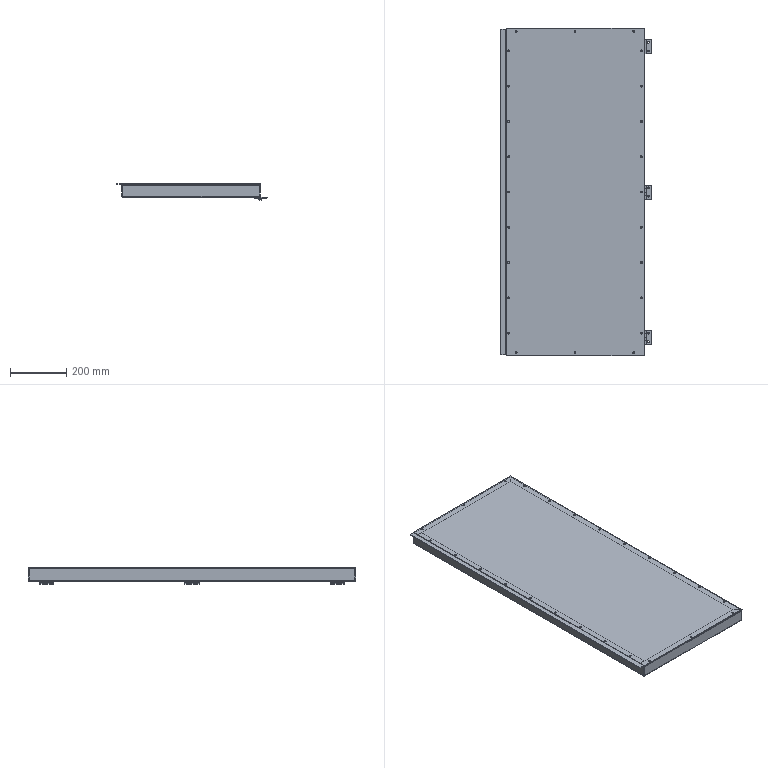Part | SolidWorks | 9 solids | 406 faces | box 537 x 1168 x 59.5 mm | volume 3187566 mm3 | cylinder 196 | plane 174 | cone 24 | spline 12 | commonest cylinder face diameters 5 x60 6.5 x48 6 x24 6.3 x24 12 x24 1.473 x8